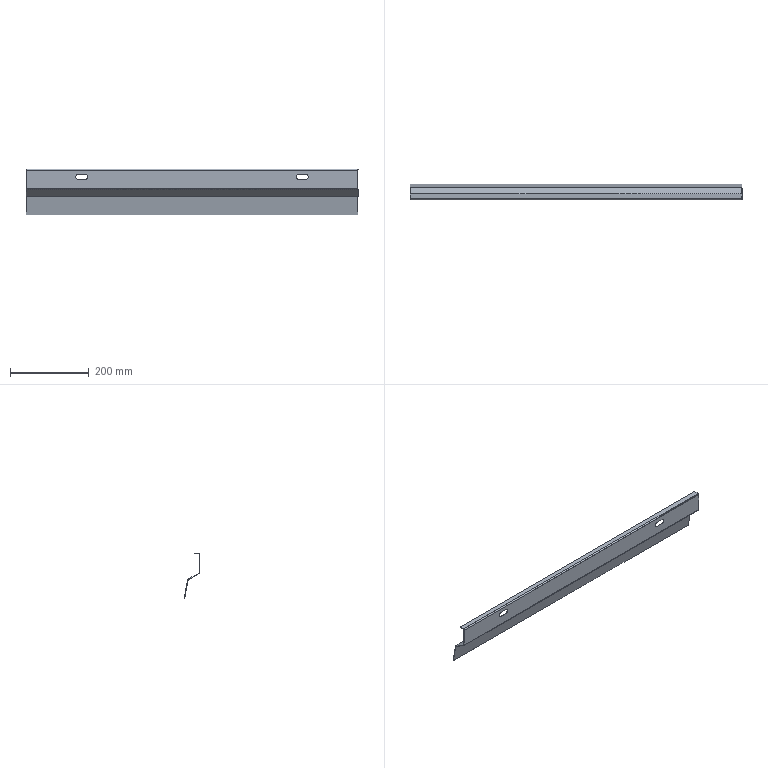Part | SolidWorks | features BaseBody 1 | 1 solid | 26 faces | box 845 x 40.182 x 116.821 mm | volume 185217 mm3 | plane 16 | cylinder 10 | commonest cylinder face diameters 13 x4 3 x3 6 x3
STEP:
#1=CARTESIAN_POINT('',(0.,37.205,-116.821));
#2=VERTEX_POINT('',#1);
#3=CARTESIAN_POINT('',(0.,28.766,-68.959));
#4=VERTEX_POINT('',#3);
#5=CARTESIAN_POINT('',(0.,25.548,-50.712));
#6=DIRECTION('',(0.,-0.1736,0.9848));
#7=VECTOR('',#6,1000.);
#8=LINE('',#5,#7);
#9=EDGE_CURVE('',#2,#4,#8,.T.);
#10=ORIENTED_EDGE('',*,*,#9,.F.);
#11=CARTESIAN_POINT('',(845.,37.205,-116.821));
#12=VERTEX_POINT('',#11);
#13=CARTESIAN_POINT('',(422.5,37.205,-116.821));
#14=DIRECTION('',(-1.,0.,0.));
#15=VECTOR('',#14,1000.);
#16=LINE('',#13,#15);
#17=EDGE_CURVE('',#12,#2,#16,.T.);
#18=ORIENTED_EDGE('',*,*,#17,.F.);
#19=CARTESIAN_POINT('',(845.,28.766,-68.959));
#20=VERTEX_POINT('',#19);
#21=CARTESIAN_POINT('',(845.,25.548,-50.712));
#22=DIRECTION('',(0.,0.1736,-0.9848));
#23=VECTOR('',#22,1000.);
#24=LINE('',#21,#23);
#25=EDGE_CURVE('',#20,#12,#24,.T.);
#26=ORIENTED_EDGE('',*,*,#25,.F.);
#27=CARTESIAN_POINT('',(422.5,28.766,-68.959));
#28=DIRECTION('',(1.,0.,0.));
#29=VECTOR('',#28,1000.);
#30=LINE('',#27,#29);
#31=EDGE_CURVE('',#4,#20,#30,.T.);
#32=ORIENTED_EDGE('',*,*,#31,.F.);
#33=EDGE_LOOP('',(#10,#18,#26,#32));
#34=FACE_OUTER_BOUND('',#33,.T.);
#35=CARTESIAN_POINT('',(422.5,25.548,-50.712));
#36=DIRECTION('',(0.,0.9848,0.1736));
#37=DIRECTION('',(0.,-0.1736,0.9848));
#38=AXIS2_PLACEMENT_3D('',#35,#36,#37);
#39=PLANE('',#38);
#40=ADVANCED_FACE('',(#34),#39,.F.);
#41=CARTESIAN_POINT('',(845.,28.038,-67.92));
#42=VERTEX_POINT('',#41);
#43=CARTESIAN_POINT('',(845.,27.288,-69.219));
#44=DIRECTION('',(-1.,0.,0.));
#45=DIRECTION('',(0.,0.,1.));
#46=AXIS2_PLACEMENT_3D('',#43,#44,#45);
#47=CIRCLE('',#46,1.5);
#48=EDGE_CURVE('',#42,#20,#47,.T.);
#49=ORIENTED_EDGE('',*,*,#48,.F.);
#50=CARTESIAN_POINT('',(0.,28.038,-67.92));
#51=VERTEX_POINT('',#50);
#52=CARTESIAN_POINT('',(422.5,28.038,-67.92));
#53=DIRECTION('',(1.,0.,0.));
#54=VECTOR('',#53,1000.);
#55=LINE('',#52,#54);
#56=EDGE_CURVE('',#51,#42,#55,.T.);
#57=ORIENTED_EDGE('',*,*,#56,.F.);
#58=CARTESIAN_POINT('',(0.,27.288,-69.219));
#59=DIRECTION('',(1.,0.,0.));
#60=DIRECTION('',(0.,0.,1.));
#61=AXIS2_PLACEMENT_3D('',#58,#59,#60);
#62=CIRCLE('',#61,1.5);
#63=EDGE_CURVE('',#4,#51,#62,.T.);
#64=ORIENTED_EDGE('',*,*,#63,.F.);
#65=ORIENTED_EDGE('',*,*,#31,.T.);
#66=EDGE_LOOP('',(#49,#57,#64,#65));
#67=FACE_OUTER_BOUND('',#66,.T.);
#68=CARTESIAN_POINT('',(422.5,27.288,-69.219));
#69=DIRECTION('',(-1.,0.,0.));
#70=DIRECTION('',(0.,0.,1.));
#71=AXIS2_PLACEMENT_3D('',#68,#69,#70);
#72=CYLINDRICAL_SURFACE('',#71,1.5);
#73=ADVANCED_FACE('',(#67),#72,.F.);
#74=CARTESIAN_POINT('',(0.,38.682,-116.561));
#75=VERTEX_POINT('',#74);
#76=CARTESIAN_POINT('',(0.,38.682,-116.561));
#77=DIRECTION('',(0.,-0.9848,-0.1736));
#78=VECTOR('',#77,1000.);
#79=LINE('',#76,#78);
#80=EDGE_CURVE('',#75,#2,#79,.T.);
#81=ORIENTED_EDGE('',*,*,#80,.T.);
#82=ORIENTED_EDGE('',*,*,#9,.T.);
#83=ORIENTED_EDGE('',*,*,#63,.T.);
#84=CARTESIAN_POINT('',(0.,0.,-51.732));
#85=VERTEX_POINT('',#84);
#86=CARTESIAN_POINT('',(0.,13.625,-59.599));
#87=DIRECTION('',(0.,-0.866,0.5));
#88=VECTOR('',#87,1000.);
#89=LINE('',#86,#88);
#90=EDGE_CURVE('',#51,#85,#89,.T.);
#91=ORIENTED_EDGE('',*,*,#90,.T.);
#92=CARTESIAN_POINT('',(0.,-1.5,-49.134));
#93=VERTEX_POINT('',#92);
#94=CARTESIAN_POINT('',(0.,1.5,-49.134));
#95=DIRECTION('',(1.,0.,0.));
#96=DIRECTION('',(0.,0.,-1.));
#97=AXIS2_PLACEMENT_3D('',#94,#95,#96);
#98=CIRCLE('',#97,3.);
#99=EDGE_CURVE('',#93,#85,#98,.T.);
#100=ORIENTED_EDGE('',*,*,#99,.F.);
#101=CARTESIAN_POINT('',(0.,-1.5,-3.));
#102=VERTEX_POINT('',#101);
#103=CARTESIAN_POINT('',(0.,-1.5,-67.129));
#104=DIRECTION('',(0.,0.,1.));
#105=VECTOR('',#104,1000.);
#106=LINE('',#103,#105);
#107=EDGE_CURVE('',#93,#102,#106,.T.);
#108=ORIENTED_EDGE('',*,*,#107,.T.);
#109=CARTESIAN_POINT('',(0.,1.5,0.));
#110=VERTEX_POINT('',#109);
#111=CARTESIAN_POINT('',(0.,1.5,-3.));
#112=DIRECTION('',(1.,0.,0.));
#113=DIRECTION('',(0.,-1.,0.));
#114=AXIS2_PLACEMENT_3D('',#111,#112,#113);
#115=CIRCLE('',#114,3.);
#116=EDGE_CURVE('',#110,#102,#115,.T.);
#117=ORIENTED_EDGE('',*,*,#116,.F.);
#118=CARTESIAN_POINT('',(0.,13.5,0.));
#119=VERTEX_POINT('',#118);
#120=CARTESIAN_POINT('',(0.,5.804,0.));
#121=DIRECTION('',(0.,1.,0.));
#122=VECTOR('',#121,1000.);
#123=LINE('',#120,#122);
#124=EDGE_CURVE('',#110,#119,#123,.T.);
#125=ORIENTED_EDGE('',*,*,#124,.T.);
#126=CARTESIAN_POINT('',(0.,13.5,-1.5));
#127=VERTEX_POINT('',#126);
#128=CARTESIAN_POINT('',(0.,13.5,-1.5));
#129=DIRECTION('',(0.,0.,1.));
#130=VECTOR('',#129,1000.);
#131=LINE('',#128,#130);
#132=EDGE_CURVE('',#127,#119,#131,.T.);
#133=ORIENTED_EDGE('',*,*,#132,.F.);
#134=CARTESIAN_POINT('',(0.,1.5,-1.5));
#135=VERTEX_POINT('',#134);
#136=CARTESIAN_POINT('',(0.,1.5,-1.5));
#137=DIRECTION('',(0.,-1.,0.));
#138=VECTOR('',#137,1000.);
#139=LINE('',#136,#138);
#140=EDGE_CURVE('',#127,#135,#139,.T.);
#141=ORIENTED_EDGE('',*,*,#140,.T.);
#142=CARTESIAN_POINT('',(0.,0.,-3.));
#143=VERTEX_POINT('',#142);
#144=CARTESIAN_POINT('',(0.,1.5,-3.));
#145=DIRECTION('',(1.,0.,0.));
#146=DIRECTION('',(0.,-1.,0.));
#147=AXIS2_PLACEMENT_3D('',#144,#145,#146);
#148=CIRCLE('',#147,1.5);
#149=EDGE_CURVE('',#135,#143,#148,.T.);
#150=ORIENTED_EDGE('',*,*,#149,.T.);
#151=CARTESIAN_POINT('',(0.,0.,-49.134));
#152=VERTEX_POINT('',#151);
#153=CARTESIAN_POINT('',(0.,0.,-85.657));
#154=DIRECTION('',(0.,0.,-1.));
#155=VECTOR('',#154,1000.);
#156=LINE('',#153,#155);
#157=EDGE_CURVE('',#143,#152,#156,.T.);
#158=ORIENTED_EDGE('',*,*,#157,.T.);
#159=CARTESIAN_POINT('',(0.,0.75,-50.433));
#160=VERTEX_POINT('',#159);
#161=CARTESIAN_POINT('',(0.,1.5,-49.134));
#162=DIRECTION('',(1.,0.,0.));
#163=DIRECTION('',(0.,0.,-1.));
#164=AXIS2_PLACEMENT_3D('',#161,#162,#163);
#165=CIRCLE('',#164,1.5);
#166=EDGE_CURVE('',#152,#160,#165,.T.);
#167=ORIENTED_EDGE('',*,*,#166,.T.);
#168=CARTESIAN_POINT('',(0.,28.788,-66.621));
#169=VERTEX_POINT('',#168);
#170=CARTESIAN_POINT('',(0.,0.75,-50.433));
#171=DIRECTION('',(0.,0.866,-0.5));
#172=VECTOR('',#171,1000.);
#173=LINE('',#170,#172);
#174=EDGE_CURVE('',#160,#169,#173,.T.);
#175=ORIENTED_EDGE('',*,*,#174,.T.);
#176=CARTESIAN_POINT('',(0.,30.243,-68.698));
#177=VERTEX_POINT('',#176);
#178=CARTESIAN_POINT('',(0.,27.288,-69.219));
#179=DIRECTION('',(1.,0.,0.));
#180=DIRECTION('',(0.,0.,1.));
#181=AXIS2_PLACEMENT_3D('',#178,#179,#180);
#182=CIRCLE('',#181,3.);
#183=EDGE_CURVE('',#177,#169,#182,.T.);
#184=ORIENTED_EDGE('',*,*,#183,.F.);
#185=CARTESIAN_POINT('',(0.,30.243,-68.698));
#186=DIRECTION('',(0.,0.1736,-0.9848));
#187=VECTOR('',#186,1000.);
#188=LINE('',#185,#187);
#189=EDGE_CURVE('',#177,#75,#188,.T.);
#190=ORIENTED_EDGE('',*,*,#189,.T.);
#191=EDGE_LOOP('',(#81,#82,#83,#91,#100,#108,#117,#125,#133,#141,#150,#158,#167,#175,#184,#190));
#192=FACE_OUTER_BOUND('',#191,.T.);
#193=CARTESIAN_POINT('',(0.,28.766,-68.959));
#194=DIRECTION('',(-1.,0.,0.));
#195=DIRECTION('',(0.,0.,1.));
#196=AXIS2_PLACEMENT_3D('',#193,#194,#195);
#197=PLANE('',#196);
#198=ADVANCED_FACE('',(#192),#197,.T.);
#199=ORIENTED_EDGE('',*,*,#17,.T.);
#200=ORIENTED_EDGE('',*,*,#80,.F.);
#201=CARTESIAN_POINT('',(845.,38.682,-116.561));
#202=VERTEX_POINT('',#201);
#203=CARTESIAN_POINT('',(0.,38.682,-116.561));
#204=DIRECTION('',(1.,0.,0.));
#205=VECTOR('',#204,1000.);
#206=LINE('',#203,#205);
#207=EDGE_CURVE('',#75,#202,#206,.T.);
#208=ORIENTED_EDGE('',*,*,#207,.T.);
#209=CARTESIAN_POINT('',(845.,37.205,-116.821));
#210=DIRECTION('',(0.,-0.9848,-0.1736));
#211=VECTOR('',#210,1000.);
#212=LINE('',#209,#211);
#213=EDGE_CURVE('',#202,#12,#212,.T.);
#214=ORIENTED_EDGE('',*,*,#213,.T.);
#215=EDGE_LOOP('',(#199,#200,#208,#214));
#216=FACE_OUTER_BOUND('',#215,.T.);
#217=CARTESIAN_POINT('',(0.,37.205,-116.821));
#218=DIRECTION('',(0.,0.1736,-0.9848));
#219=DIRECTION('',(0.,0.9848,0.1736));
#220=AXIS2_PLACEMENT_3D('',#217,#218,#219);
#221=PLANE('',#220);
#222=ADVANCED_FACE('',(#216),#221,.T.);
#223=ORIENTED_EDGE('',*,*,#213,.F.);
#224=CARTESIAN_POINT('',(845.,30.243,-68.698));
#225=VERTEX_POINT('',#224);
#226=CARTESIAN_POINT('',(845.,38.682,-116.561));
#227=DIRECTION('',(0.,-0.1736,0.9848));
#228=VECTOR('',#227,1000.);
#229=LINE('',#226,#228);
#230=EDGE_CURVE('',#202,#225,#229,.T.);
#231=ORIENTED_EDGE('',*,*,#230,.T.);
#232=CARTESIAN_POINT('',(845.,28.788,-66.621));
#233=VERTEX_POINT('',#232);
#234=CARTESIAN_POINT('',(845.,27.288,-69.219));
#235=DIRECTION('',(-1.,0.,0.));
#236=DIRECTION('',(0.,0.,1.));
#237=AXIS2_PLACEMENT_3D('',#234,#235,#236);
#238=CIRCLE('',#237,3.);
#239=EDGE_CURVE('',#233,#225,#238,.T.);
#240=ORIENTED_EDGE('',*,*,#239,.F.);
#241=CARTESIAN_POINT('',(845.,0.75,-50.433));
#242=VERTEX_POINT('',#241);
#243=CARTESIAN_POINT('',(845.,28.788,-66.621));
#244=DIRECTION('',(0.,-0.866,0.5));
#245=VECTOR('',#244,1000.);
#246=LINE('',#243,#245);
#247=EDGE_CURVE('',#233,#242,#246,.T.);
#248=ORIENTED_EDGE('',*,*,#247,.T.);
#249=CARTESIAN_POINT('',(845.,0.,-49.134));
#250=VERTEX_POINT('',#249);
#251=CARTESIAN_POINT('',(845.,1.5,-49.134));
#252=DIRECTION('',(-1.,0.,0.));
#253=DIRECTION('',(0.,0.,-1.));
#254=AXIS2_PLACEMENT_3D('',#251,#252,#253);
#255=CIRCLE('',#254,1.5);
#256=EDGE_CURVE('',#242,#250,#255,.T.);
#257=ORIENTED_EDGE('',*,*,#256,.T.);
#258=CARTESIAN_POINT('',(845.,0.,-3.));
#259=VERTEX_POINT('',#258);
#260=CARTESIAN_POINT('',(845.,0.,-49.134));
#261=DIRECTION('',(0.,0.,1.));
#262=VECTOR('',#261,1000.);
#263=LINE('',#260,#262);
#264=EDGE_CURVE('',#250,#259,#263,.T.);
#265=ORIENTED_EDGE('',*,*,#264,.T.);
#266=CARTESIAN_POINT('',(845.,1.5,-1.5));
#267=VERTEX_POINT('',#266);
#268=CARTESIAN_POINT('',(845.,1.5,-3.));
#269=DIRECTION('',(-1.,0.,0.));
#270=DIRECTION('',(0.,-1.,0.));
#271=AXIS2_PLACEMENT_3D('',#268,#269,#270);
#272=CIRCLE('',#271,1.5);
#273=EDGE_CURVE('',#259,#267,#272,.T.);
#274=ORIENTED_EDGE('',*,*,#273,.T.);
#275=CARTESIAN_POINT('',(845.,13.5,-1.5));
#276=VERTEX_POINT('',#275);
#277=CARTESIAN_POINT('',(845.,1.5,-1.5));
#278=DIRECTION('',(0.,1.,0.));
#279=VECTOR('',#278,1000.);
#280=LINE('',#277,#279);
#281=EDGE_CURVE('',#267,#276,#280,.T.);
#282=ORIENTED_EDGE('',*,*,#281,.T.);
#283=CARTESIAN_POINT('',(845.,13.5,0.));
#284=VERTEX_POINT('',#283);
#285=CARTESIAN_POINT('',(845.,13.5,-1.5));
#286=DIRECTION('',(0.,0.,1.));
#287=VECTOR('',#286,1000.);
#288=LINE('',#285,#287);
#289=EDGE_CURVE('',#276,#284,#288,.T.);
#290=ORIENTED_EDGE('',*,*,#289,.T.);
#291=CARTESIAN_POINT('',(845.,1.5,0.));
#292=VERTEX_POINT('',#291);
#293=CARTESIAN_POINT('',(845.,5.804,0.));
#294=DIRECTION('',(0.,-1.,0.));
#295=VECTOR('',#294,1000.);
#296=LINE('',#293,#295);
#297=EDGE_CURVE('',#284,#292,#296,.T.);
#298=ORIENTED_EDGE('',*,*,#297,.T.);
#299=CARTESIAN_POINT('',(845.,-1.5,-3.));
#300=VERTEX_POINT('',#299);
#301=CARTESIAN_POINT('',(845.,1.5,-3.));
#302=DIRECTION('',(-1.,0.,0.));
#303=DIRECTION('',(0.,-1.,0.));
#304=AXIS2_PLACEMENT_3D('',#301,#302,#303);
#305=CIRCLE('',#304,3.);
#306=EDGE_CURVE('',#300,#292,#305,.T.);
#307=ORIENTED_EDGE('',*,*,#306,.F.);
#308=CARTESIAN_POINT('',(845.,-1.5,-49.134));
#309=VERTEX_POINT('',#308);
#310=CARTESIAN_POINT('',(845.,-1.5,-67.129));
#311=DIRECTION('',(0.,0.,-1.));
#312=VECTOR('',#311,1000.);
#313=LINE('',#310,#312);
#314=EDGE_CURVE('',#300,#309,#313,.T.);
#315=ORIENTED_EDGE('',*,*,#314,.T.);
#316=CARTESIAN_POINT('',(845.,0.,-51.732));
#317=VERTEX_POINT('',#316);
#318=CARTESIAN_POINT('',(845.,1.5,-49.134));
#319=DIRECTION('',(-1.,0.,0.));
#320=DIRECTION('',(0.,0.,-1.));
#321=AXIS2_PLACEMENT_3D('',#318,#319,#320);
#322=CIRCLE('',#321,3.);
#323=EDGE_CURVE('',#317,#309,#322,.T.);
#324=ORIENTED_EDGE('',*,*,#323,.F.);
#325=CARTESIAN_POINT('',(845.,13.625,-59.599));
#326=DIRECTION('',(0.,0.866,-0.5));
#327=VECTOR('',#326,1000.);
#328=LINE('',#325,#327);
#329=EDGE_CURVE('',#317,#42,#328,.T.);
#330=ORIENTED_EDGE('',*,*,#329,.T.);
#331=ORIENTED_EDGE('',*,*,#48,.T.);
#332=ORIENTED_EDGE('',*,*,#25,.T.);
#333=EDGE_LOOP('',(#223,#231,#240,#248,#257,#265,#274,#282,#290,#298,#307,#315,#324,#330,#331,#332));
#334=FACE_OUTER_BOUND('',#333,.T.);
#335=CARTESIAN_POINT('',(845.,22.424,-32.991));
#336=DIRECTION('',(1.,0.,0.));
#337=DIRECTION('',(0.,0.,-1.));
#338=AXIS2_PLACEMENT_3D('',#335,#336,#337);
#339=PLANE('',#338);
#340=ADVANCED_FACE('',(#334),#339,.T.);
#341=ORIENTED_EDGE('',*,*,#329,.F.);
#342=CARTESIAN_POINT('',(422.5,0.,-51.732));
#343=DIRECTION('',(1.,0.,0.));
#344=VECTOR('',#343,1000.);
#345=LINE('',#342,#344);
#346=EDGE_CURVE('',#85,#317,#345,.T.);
#347=ORIENTED_EDGE('',*,*,#346,.F.);
#348=ORIENTED_EDGE('',*,*,#90,.F.);
#349=ORIENTED_EDGE('',*,*,#56,.T.);
#350=EDGE_LOOP('',(#341,#347,#348,#349));
#351=FACE_OUTER_BOUND('',#350,.T.);
#352=CARTESIAN_POINT('',(422.5,13.625,-59.599));
#353=DIRECTION('',(0.,0.5,0.866));
#354=DIRECTION('',(0.,-0.866,0.5));
#355=AXIS2_PLACEMENT_3D('',#352,#353,#354);
#356=PLANE('',#355);
#357=ADVANCED_FACE('',(#351),#356,.F.);
#358=ORIENTED_EDGE('',*,*,#207,.F.);
#359=ORIENTED_EDGE('',*,*,#189,.F.);
#360=CARTESIAN_POINT('',(422.5,30.243,-68.698));
#361=DIRECTION('',(1.,0.,0.));
#362=VECTOR('',#361,1000.);
#363=LINE('',#360,#362);
#364=EDGE_CURVE('',#177,#225,#363,.T.);
#365=ORIENTED_EDGE('',*,*,#364,.T.);
#366=ORIENTED_EDGE('',*,*,#230,.F.);
#367=EDGE_LOOP('',(#358,#359,#365,#366));
#368=FACE_OUTER_BOUND('',#367,.T.);
#369=CARTESIAN_POINT('',(422.5,27.026,-50.452));
#370=DIRECTION('',(0.,0.9848,0.1736));
#371=DIRECTION('',(0.,-0.1736,0.9848));
#372=AXIS2_PLACEMENT_3D('',#369,#370,#371);
#373=PLANE('',#372);
#374=ADVANCED_FACE('',(#368),#373,.T.);
#375=CARTESIAN_POINT('',(422.5,-1.5,-49.134));
#376=DIRECTION('',(-1.,0.,0.));
#377=VECTOR('',#376,1000.);
#378=LINE('',#375,#377);
#379=EDGE_CURVE('',#309,#93,#378,.T.);
#380=ORIENTED_EDGE('',*,*,#379,.T.);
#381=ORIENTED_EDGE('',*,*,#99,.T.);
#382=ORIENTED_EDGE('',*,*,#346,.T.);
#383=ORIENTED_EDGE('',*,*,#323,.T.);
#384=EDGE_LOOP('',(#380,#381,#382,#383));
#385=FACE_OUTER_BOUND('',#384,.T.);
#386=CARTESIAN_POINT('',(422.5,1.5,-49.134));
#387=DIRECTION('',(1.,0.,0.));
#388=DIRECTION('',(0.,0.,-1.));
#389=AXIS2_PLACEMENT_3D('',#386,#387,#388);
#390=CYLINDRICAL_SURFACE('',#389,3.);
#391=ADVANCED_FACE('',(#385),#390,.T.);
#392=CARTESIAN_POINT('',(422.5,28.788,-66.621));
#393=DIRECTION('',(1.,0.,0.));
#394=VECTOR('',#393,1000.);
#395=LINE('',#392,#394);
#396=EDGE_CURVE('',#169,#233,#395,.T.);
#397=ORIENTED_EDGE('',*,*,#396,.T.);
#398=ORIENTED_EDGE('',*,*,#239,.T.);
#399=ORIENTED_EDGE('',*,*,#364,.F.);
#400=ORIENTED_EDGE('',*,*,#183,.T.);
#401=EDGE_LOOP('',(#397,#398,#399,#400));
#402=FACE_OUTER_BOUND('',#401,.T.);
#403=CARTESIAN_POINT('',(422.5,27.288,-69.219));
#404=DIRECTION('',(-1.,0.,0.));
#405=DIRECTION('',(0.,0.,1.));
#406=AXIS2_PLACEMENT_3D('',#403,#404,#405);
#407=CYLINDRICAL_SURFACE('',#406,3.);
#408=ADVANCED_FACE('',(#402),#407,.T.);
#409=CARTESIAN_POINT('',(422.5,0.75,-50.433));
#410=DIRECTION('',(1.,0.,0.));
#411=VECTOR('',#410,1000.);
#412=LINE('',#409,#411);
#413=EDGE_CURVE('',#160,#242,#412,.T.);
#414=ORIENTED_EDGE('',*,*,#413,.T.);
#415=ORIENTED_EDGE('',*,*,#247,.F.);
#416=ORIENTED_EDGE('',*,*,#396,.F.);
#417=ORIENTED_EDGE('',*,*,#174,.F.);
#418=EDGE_LOOP('',(#414,#415,#416,#417));
#419=FACE_OUTER_BOUND('',#418,.T.);
#420=CARTESIAN_POINT('',(422.5,14.375,-58.3));
#421=DIRECTION('',(0.,0.5,0.866));
#422=DIRECTION('',(0.,-0.866,0.5));
#423=AXIS2_PLACEMENT_3D('',#420,#421,#422);
#424=PLANE('',#423);
#425=ADVANCED_FACE('',(#419),#424,.T.);
#426=CARTESIAN_POINT('',(695.,-1.5,-26.5));
#427=VERTEX_POINT('',#426);
#428=CARTESIAN_POINT('',(712.,-1.5,-26.5));
#429=VERTEX_POINT('',#428);
#430=CARTESIAN_POINT('',(422.5,-1.5,-26.5));
#431=DIRECTION('',(1.,0.,0.));
#432=VECTOR('',#431,1000.);
#433=LINE('',#430,#432);
#434=EDGE_CURVE('',#427,#429,#433,.T.);
#435=ORIENTED_EDGE('',*,*,#434,.F.);
#436=CARTESIAN_POINT('',(695.,-1.5,-13.5));
#437=VERTEX_POINT('',#436);
#438=CARTESIAN_POINT('',(695.,-1.5,-20.));
#439=DIRECTION('',(0.,-1.,0.));
#440=DIRECTION('',(0.,0.,1.));
#441=AXIS2_PLACEMENT_3D('',#438,#439,#440);
#442=CIRCLE('',#441,6.5);
#443=EDGE_CURVE('',#437,#427,#442,.T.);
#444=ORIENTED_EDGE('',*,*,#443,.F.);
#445=CARTESIAN_POINT('',(712.,-1.5,-13.5));
#446=VERTEX_POINT('',#445);
#447=CARTESIAN_POINT('',(422.5,-1.5,-13.5));
#448=DIRECTION('',(-1.,0.,0.));
#449=VECTOR('',#448,1000.);
#450=LINE('',#447,#449);
#451=EDGE_CURVE('',#446,#437,#450,.T.);
#452=ORIENTED_EDGE('',*,*,#451,.F.);
#453=CARTESIAN_POINT('',(712.,-1.5,-20.));
#454=DIRECTION('',(0.,-1.,0.));
#455=DIRECTION('',(0.,0.,1.));
#456=AXIS2_PLACEMENT_3D('',#453,#454,#455);
#457=CIRCLE('',#456,6.5);
#458=EDGE_CURVE('',#429,#446,#457,.T.);
#459=ORIENTED_EDGE('',*,*,#458,.F.);
#460=EDGE_LOOP('',(#435,#444,#452,#459));
#461=FACE_BOUND('',#460,.T.);
#462=CARTESIAN_POINT('',(133.,-1.5,-26.5));
#463=VERTEX_POINT('',#462);
#464=CARTESIAN_POINT('',(150.,-1.5,-26.5));
#465=VERTEX_POINT('',#464);
#466=CARTESIAN_POINT('',(422.5,-1.5,-26.5));
#467=DIRECTION('',(1.,0.,0.));
#468=VECTOR('',#467,1000.);
#469=LINE('',#466,#468);
#470=EDGE_CURVE('',#463,#465,#469,.T.);
#471=ORIENTED_EDGE('',*,*,#470,.F.);
#472=CARTESIAN_POINT('',(133.,-1.5,-13.5));
#473=VERTEX_POINT('',#472);
#474=CARTESIAN_POINT('',(133.,-1.5,-20.));
#475=DIRECTION('',(0.,-1.,0.));
#476=DIRECTION('',(0.,0.,1.));
#477=AXIS2_PLACEMENT_3D('',#474,#475,#476);
#478=CIRCLE('',#477,6.5);
#479=EDGE_CURVE('',#473,#463,#478,.T.);
#480=ORIENTED_EDGE('',*,*,#479,.F.);
#481=CARTESIAN_POINT('',(150.,-1.5,-13.5));
#482=VERTEX_POINT('',#481);
#483=CARTESIAN_POINT('',(422.5,-1.5,-13.5));
#484=DIRECTION('',(-1.,0.,0.));
#485=VECTOR('',#484,1000.);
#486=LINE('',#483,#485);
#487=EDGE_CURVE('',#482,#473,#486,.T.);
#488=ORIENTED_EDGE('',*,*,#487,.F.);
#489=CARTESIAN_POINT('',(150.,-1.5,-20.));
#490=DIRECTION('',(0.,-1.,0.));
#491=DIRECTION('',(0.,0.,1.));
#492=AXIS2_PLACEMENT_3D('',#489,#490,#491);
#493=CIRCLE('',#492,6.5);
#494=EDGE_CURVE('',#465,#482,#493,.T.);
#495=ORIENTED_EDGE('',*,*,#494,.F.);
#496=EDGE_LOOP('',(#471,#480,#488,#495));
#497=FACE_BOUND('',#496,.T.);
#498=ORIENTED_EDGE('',*,*,#107,.F.);
#499=ORIENTED_EDGE('',*,*,#379,.F.);
#500=ORIENTED_EDGE('',*,*,#314,.F.);
#501=CARTESIAN_POINT('',(422.5,-1.5,-3.));
#502=DIRECTION('',(1.,0.,0.));
#503=VECTOR('',#502,1000.);
#504=LINE('',#501,#503);
#505=EDGE_CURVE('',#102,#300,#504,.T.);
#506=ORIENTED_EDGE('',*,*,#505,.F.);
#507=EDGE_LOOP('',(#498,#499,#500,#506));
#508=FACE_OUTER_BOUND('',#507,.T.);
#509=CARTESIAN_POINT('',(422.5,-1.5,-67.129));
#510=DIRECTION('',(0.,1.,0.));
#511=DIRECTION('',(0.,0.,1.));
#512=AXIS2_PLACEMENT_3D('',#509,#510,#511);
#513=PLANE('',#512);
#514=ADVANCED_FACE('',(#461,#497,#508),#513,.F.);
#515=ORIENTED_EDGE('',*,*,#166,.F.);
#516=CARTESIAN_POINT('',(422.5,0.,-49.134));
#517=DIRECTION('',(-1.,0.,0.));
#518=VECTOR('',#517,1000.);
#519=LINE('',#516,#518);
#520=EDGE_CURVE('',#250,#152,#519,.T.);
#521=ORIENTED_EDGE('',*,*,#520,.F.);
#522=ORIENTED_EDGE('',*,*,#256,.F.);
#523=ORIENTED_EDGE('',*,*,#413,.F.);
#524=EDGE_LOOP('',(#515,#521,#522,#523));
#525=FACE_OUTER_BOUND('',#524,.T.);
#526=CARTESIAN_POINT('',(422.5,1.5,-49.134));
#527=DIRECTION('',(1.,0.,0.));
#528=DIRECTION('',(0.,0.,-1.));
#529=AXIS2_PLACEMENT_3D('',#526,#527,#528);
#530=CYLINDRICAL_SURFACE('',#529,1.5);
#531=ADVANCED_FACE('',(#525),#530,.F.);
#532=CARTESIAN_POINT('',(712.,0.,-13.5));
#533=VERTEX_POINT('',#532);
#534=CARTESIAN_POINT('',(712.,-1.5,-13.5));
#535=DIRECTION('',(0.,-1.,0.));
#536=VECTOR('',#535,1000.);
#537=LINE('',#534,#536);
#538=EDGE_CURVE('',#533,#446,#537,.T.);
#539=ORIENTED_EDGE('',*,*,#538,.F.);
#540=CARTESIAN_POINT('',(712.,0.,-26.5));
#541=VERTEX_POINT('',#540);
#542=CARTESIAN_POINT('',(712.,0.,-20.));
#543=DIRECTION('',(0.,-1.,0.));
#544=DIRECTION('',(0.,0.,1.));
#545=AXIS2_PLACEMENT_3D('',#542,#543,#544);
#546=CIRCLE('',#545,6.5);
#547=EDGE_CURVE('',#541,#533,#546,.T.);
#548=ORIENTED_EDGE('',*,*,#547,.F.);
#549=CARTESIAN_POINT('',(712.,-1.5,-26.5));
#550=DIRECTION('',(0.,1.,0.));
#551=VECTOR('',#550,1000.);
#552=LINE('',#549,#551);
#553=EDGE_CURVE('',#429,#541,#552,.T.);
#554=ORIENTED_EDGE('',*,*,#553,.F.);
#555=ORIENTED_EDGE('',*,*,#458,.T.);
#556=EDGE_LOOP('',(#539,#548,#554,#555));
#557=FACE_OUTER_BOUND('',#556,.T.);
#558=CARTESIAN_POINT('',(712.,-1.5,-20.));
#559=DIRECTION('',(0.,1.,0.));
#560=DIRECTION('',(0.,0.,1.));
#561=AXIS2_PLACEMENT_3D('',#558,#559,#560);
#562=CYLINDRICAL_SURFACE('',#561,6.5);
#563=ADVANCED_FACE('',(#557),#562,.F.);
#564=ORIENTED_EDGE('',*,*,#553,.T.);
#565=CARTESIAN_POINT('',(695.,0.,-26.5));
#566=VERTEX_POINT('',#565);
#567=CARTESIAN_POINT('',(712.,0.,-26.5));
#568=DIRECTION('',(1.,0.,0.));
#569=VECTOR('',#568,1000.);
#570=LINE('',#567,#569);
#571=EDGE_CURVE('',#566,#541,#570,.T.);
#572=ORIENTED_EDGE('',*,*,#571,.F.);
#573=CARTESIAN_POINT('',(695.,-1.5,-26.5));
#574=DIRECTION('',(0.,1.,0.));
#575=VECTOR('',#574,1000.);
#576=LINE('',#573,#575);
#577=EDGE_CURVE('',#427,#566,#576,.T.);
#578=ORIENTED_EDGE('',*,*,#577,.F.);
#579=ORIENTED_EDGE('',*,*,#434,.T.);
#580=EDGE_LOOP('',(#564,#572,#578,#579));
#581=FACE_OUTER_BOUND('',#580,.T.);
#582=CARTESIAN_POINT('',(712.,-1.5,-26.5));
#583=DIRECTION('',(0.,0.,-1.));
#584=DIRECTION('',(-1.,0.,0.));
#585=AXIS2_PLACEMENT_3D('',#582,#583,#584);
#586=PLANE('',#585);
#587=ADVANCED_FACE('',(#581),#586,.F.);
#588=ORIENTED_EDGE('',*,*,#577,.T.);
#589=CARTESIAN_POINT('',(695.,0.,-13.5));
#590=VERTEX_POINT('',#589);
#591=CARTESIAN_POINT('',(695.,0.,-20.));
#592=DIRECTION('',(0.,-1.,0.));
#593=DIRECTION('',(0.,0.,1.));
#594=AXIS2_PLACEMENT_3D('',#591,#592,#593);
#595=CIRCLE('',#594,6.5);
#596=EDGE_CURVE('',#590,#566,#595,.T.);
#597=ORIENTED_EDGE('',*,*,#596,.F.);
#598=CARTESIAN_POINT('',(695.,-1.5,-13.5));
#599=DIRECTION('',(0.,1.,0.));
#600=VECTOR('',#599,1000.);
#601=LINE('',#598,#600);
#602=EDGE_CURVE('',#437,#590,#601,.T.);
#603=ORIENTED_EDGE('',*,*,#602,.F.);
#604=ORIENTED_EDGE('',*,*,#443,.T.);
#605=EDGE_LOOP('',(#588,#597,#603,#604));
#606=FACE_OUTER_BOUND('',#605,.T.);
#607=CARTESIAN_POINT('',(695.,-1.5,-20.));
#608=DIRECTION('',(0.,1.,0.));
#609=DIRECTION('',(0.,0.,1.));
#610=AXIS2_PLACEMENT_3D('',#607,#608,#609);
#611=CYLINDRICAL_SURFACE('',#610,6.5);
#612=ADVANCED_FACE('',(#606),#611,.F.);
#613=ORIENTED_EDGE('',*,*,#602,.T.);
#614=CARTESIAN_POINT('',(695.,0.,-13.5));
#615=DIRECTION('',(-1.,0.,0.));
#616=VECTOR('',#615,1000.);
#617=LINE('',#614,#616);
#618=EDGE_CURVE('',#533,#590,#617,.T.);
#619=ORIENTED_EDGE('',*,*,#618,.F.);
#620=ORIENTED_EDGE('',*,*,#538,.T.);
#621=ORIENTED_EDGE('',*,*,#451,.T.);
#622=EDGE_LOOP('',(#613,#619,#620,#621));
#623=FACE_OUTER_BOUND('',#622,.T.);
#624=CARTESIAN_POINT('',(695.,-1.5,-13.5));
#625=DIRECTION('',(0.,0.,1.));
#626=DIRECTION('',(1.,0.,0.));
#627=AXIS2_PLACEMENT_3D('',#624,#625,#626);
#628=PLANE('',#627);
#629=ADVANCED_FACE('',(#623),#628,.F.);
#630=CARTESIAN_POINT('',(150.,0.,-13.5));
#631=VERTEX_POINT('',#630);
#632=CARTESIAN_POINT('',(150.,-1.5,-13.5));
#633=DIRECTION('',(0.,-1.,0.));
#634=VECTOR('',#633,1000.);
#635=LINE('',#632,#634);
#636=EDGE_CURVE('',#631,#482,#635,.T.);
#637=ORIENTED_EDGE('',*,*,#636,.F.);
#638=CARTESIAN_POINT('',(150.,0.,-26.5));
#639=VERTEX_POINT('',#638);
#640=CARTESIAN_POINT('',(150.,0.,-20.));
#641=DIRECTION('',(0.,-1.,0.));
#642=DIRECTION('',(0.,0.,1.));
#643=AXIS2_PLACEMENT_3D('',#640,#641,#642);
#644=CIRCLE('',#643,6.5);
#645=EDGE_CURVE('',#639,#631,#644,.T.);
#646=ORIENTED_EDGE('',*,*,#645,.F.);
#647=CARTESIAN_POINT('',(150.,-1.5,-26.5));
#648=DIRECTION('',(0.,1.,0.));
#649=VECTOR('',#648,1000.);
#650=LINE('',#647,#649);
#651=EDGE_CURVE('',#465,#639,#650,.T.);
#652=ORIENTED_EDGE('',*,*,#651,.F.);
#653=ORIENTED_EDGE('',*,*,#494,.T.);
#654=EDGE_LOOP('',(#637,#646,#652,#653));
#655=FACE_OUTER_BOUND('',#654,.T.);
#656=CARTESIAN_POINT('',(150.,-1.5,-20.));
#657=DIRECTION('',(0.,1.,0.));
#658=DIRECTION('',(0.,0.,1.));
#659=AXIS2_PLACEMENT_3D('',#656,#657,#658);
#660=CYLINDRICAL_SURFACE('',#659,6.5);
#661=ADVANCED_FACE('',(#655),#660,.F.);
#662=ORIENTED_EDGE('',*,*,#651,.T.);
#663=CARTESIAN_POINT('',(133.,0.,-26.5));
#664=VERTEX_POINT('',#663);
#665=CARTESIAN_POINT('',(150.,0.,-26.5));
#666=DIRECTION('',(1.,0.,0.));
#667=VECTOR('',#666,1000.);
#668=LINE('',#665,#667);
#669=EDGE_CURVE('',#664,#639,#668,.T.);
#670=ORIENTED_EDGE('',*,*,#669,.F.);
#671=CARTESIAN_POINT('',(133.,-1.5,-26.5));
#672=DIRECTION('',(0.,1.,0.));
#673=VECTOR('',#672,1000.);
#674=LINE('',#671,#673);
#675=EDGE_CURVE('',#463,#664,#674,.T.);
#676=ORIENTED_EDGE('',*,*,#675,.F.);
#677=ORIENTED_EDGE('',*,*,#470,.T.);
#678=EDGE_LOOP('',(#662,#670,#676,#677));
#679=FACE_OUTER_BOUND('',#678,.T.);
#680=CARTESIAN_POINT('',(150.,-1.5,-26.5));
#681=DIRECTION('',(0.,0.,-1.));
#682=DIRECTION('',(-1.,0.,0.));
#683=AXIS2_PLACEMENT_3D('',#680,#681,#682);
#684=PLANE('',#683);
#685=ADVANCED_FACE('',(#679),#684,.F.);
#686=ORIENTED_EDGE('',*,*,#675,.T.);
#687=CARTESIAN_POINT('',(133.,0.,-13.5));
#688=VERTEX_POINT('',#687);
#689=CARTESIAN_POINT('',(133.,0.,-20.));
#690=DIRECTION('',(0.,-1.,0.));
#691=DIRECTION('',(0.,0.,1.));
#692=AXIS2_PLACEMENT_3D('',#689,#690,#691);
#693=CIRCLE('',#692,6.5);
#694=EDGE_CURVE('',#688,#664,#693,.T.);
#695=ORIENTED_EDGE('',*,*,#694,.F.);
#696=CARTESIAN_POINT('',(133.,-1.5,-13.5));
#697=DIRECTION('',(0.,1.,0.));
#698=VECTOR('',#697,1000.);
#699=LINE('',#696,#698);
#700=EDGE_CURVE('',#473,#688,#699,.T.);
#701=ORIENTED_EDGE('',*,*,#700,.F.);
#702=ORIENTED_EDGE('',*,*,#479,.T.);
#703=EDGE_LOOP('',(#686,#695,#701,#702));
#704=FACE_OUTER_BOUND('',#703,.T.);
#705=CARTESIAN_POINT('',(133.,-1.5,-20.));
#706=DIRECTION('',(0.,1.,0.));
#707=DIRECTION('',(0.,0.,1.));
#708=AXIS2_PLACEMENT_3D('',#705,#706,#707);
#709=CYLINDRICAL_SURFACE('',#708,6.5);
#710=ADVANCED_FACE('',(#704),#709,.F.);
#711=ORIENTED_EDGE('',*,*,#700,.T.);
#712=CARTESIAN_POINT('',(133.,0.,-13.5));
#713=DIRECTION('',(-1.,0.,0.));
#714=VECTOR('',#713,1000.);
#715=LINE('',#712,#714);
#716=EDGE_CURVE('',#631,#688,#715,.T.);
#717=ORIENTED_EDGE('',*,*,#716,.F.);
#718=ORIENTED_EDGE('',*,*,#636,.T.);
#719=ORIENTED_EDGE('',*,*,#487,.T.);
#720=EDGE_LOOP('',(#711,#717,#718,#719));
#721=FACE_OUTER_BOUND('',#720,.T.);
#722=CARTESIAN_POINT('',(133.,-1.5,-13.5));
#723=DIRECTION('',(0.,0.,1.));
#724=DIRECTION('',(1.,0.,0.));
#725=AXIS2_PLACEMENT_3D('',#722,#723,#724);
#726=PLANE('',#725);
#727=ADVANCED_FACE('',(#721),#726,.F.);
#728=ORIENTED_EDGE('',*,*,#505,.T.);
#729=ORIENTED_EDGE('',*,*,#306,.T.);
#730=CARTESIAN_POINT('',(422.5,1.5,0.));
#731=DIRECTION('',(-1.,0.,0.));
#732=VECTOR('',#731,1000.);
#733=LINE('',#730,#732);
#734=EDGE_CURVE('',#292,#110,#733,.T.);
#735=ORIENTED_EDGE('',*,*,#734,.T.);
#736=ORIENTED_EDGE('',*,*,#116,.T.);
#737=EDGE_LOOP('',(#728,#729,#735,#736));
#738=FACE_OUTER_BOUND('',#737,.T.);
#739=CARTESIAN_POINT('',(422.5,1.5,-3.));
#740=DIRECTION('',(-1.,0.,0.));
#741=DIRECTION('',(0.,-1.,0.));
#742=AXIS2_PLACEMENT_3D('',#739,#740,#741);
#743=CYLINDRICAL_SURFACE('',#742,3.);
#744=ADVANCED_FACE('',(#738),#743,.T.);
#745=ORIENTED_EDGE('',*,*,#596,.T.);
#746=ORIENTED_EDGE('',*,*,#571,.T.);
#747=ORIENTED_EDGE('',*,*,#547,.T.);
#748=ORIENTED_EDGE('',*,*,#618,.T.);
#749=EDGE_LOOP('',(#745,#746,#747,#748));
#750=FACE_BOUND('',#749,.T.);
#751=ORIENTED_EDGE('',*,*,#694,.T.);
#752=ORIENTED_EDGE('',*,*,#669,.T.);
#753=ORIENTED_EDGE('',*,*,#645,.T.);
#754=ORIENTED_EDGE('',*,*,#716,.T.);
#755=EDGE_LOOP('',(#751,#752,#753,#754));
#756=FACE_BOUND('',#755,.T.);
#757=ORIENTED_EDGE('',*,*,#520,.T.);
#758=ORIENTED_EDGE('',*,*,#157,.F.);
#759=CARTESIAN_POINT('',(422.5,0.,-3.));
#760=DIRECTION('',(1.,0.,0.));
#761=VECTOR('',#760,1000.);
#762=LINE('',#759,#761);
#763=EDGE_CURVE('',#143,#259,#762,.T.);
#764=ORIENTED_EDGE('',*,*,#763,.T.);
#765=ORIENTED_EDGE('',*,*,#264,.F.);
#766=EDGE_LOOP('',(#757,#758,#764,#765));
#767=FACE_OUTER_BOUND('',#766,.T.);
#768=CARTESIAN_POINT('',(422.5,0.,-67.129));
#769=DIRECTION('',(0.,1.,0.));
#770=DIRECTION('',(0.,0.,1.));
#771=AXIS2_PLACEMENT_3D('',#768,#769,#770);
#772=PLANE('',#771);
#773=ADVANCED_FACE('',(#750,#756,#767),#772,.T.);
#774=ORIENTED_EDGE('',*,*,#297,.F.);
#775=CARTESIAN_POINT('',(422.5,13.5,0.));
#776=DIRECTION('',(1.,0.,0.));
#777=VECTOR('',#776,1000.);
#778=LINE('',#775,#777);
#779=EDGE_CURVE('',#119,#284,#778,.T.);
#780=ORIENTED_EDGE('',*,*,#779,.F.);
#781=ORIENTED_EDGE('',*,*,#124,.F.);
#782=ORIENTED_EDGE('',*,*,#734,.F.);
#783=EDGE_LOOP('',(#774,#780,#781,#782));
#784=FACE_OUTER_BOUND('',#783,.T.);
#785=CARTESIAN_POINT('',(422.5,5.804,0.));
#786=DIRECTION('',(0.,0.,-1.));
#787=DIRECTION('',(0.,1.,0.));
#788=AXIS2_PLACEMENT_3D('',#785,#786,#787);
#789=PLANE('',#788);
#790=ADVANCED_FACE('',(#784),#789,.F.);
#791=ORIENTED_EDGE('',*,*,#273,.F.);
#792=ORIENTED_EDGE('',*,*,#763,.F.);
#793=ORIENTED_EDGE('',*,*,#149,.F.);
#794=CARTESIAN_POINT('',(422.5,1.5,-1.5));
#795=DIRECTION('',(-1.,0.,0.));
#796=VECTOR('',#795,1000.);
#797=LINE('',#794,#796);
#798=EDGE_CURVE('',#267,#135,#797,.T.);
#799=ORIENTED_EDGE('',*,*,#798,.F.);
#800=EDGE_LOOP('',(#791,#792,#793,#799));
#801=FACE_OUTER_BOUND('',#800,.T.);
#802=CARTESIAN_POINT('',(422.5,1.5,-3.));
#803=DIRECTION('',(-1.,0.,0.));
#804=DIRECTION('',(0.,-1.,0.));
#805=AXIS2_PLACEMENT_3D('',#802,#803,#804);
#806=CYLINDRICAL_SURFACE('',#805,1.5);
#807=ADVANCED_FACE('',(#801),#806,.F.);
#808=CARTESIAN_POINT('',(0.,13.5,-1.5));
#809=DIRECTION('',(-1.,0.,0.));
#810=VECTOR('',#809,1000.);
#811=LINE('',#808,#810);
#812=EDGE_CURVE('',#276,#127,#811,.T.);
#813=ORIENTED_EDGE('',*,*,#812,.T.);
#814=ORIENTED_EDGE('',*,*,#132,.T.);
#815=ORIENTED_EDGE('',*,*,#779,.T.);
#816=ORIENTED_EDGE('',*,*,#289,.F.);
#817=EDGE_LOOP('',(#813,#814,#815,#816));
#818=FACE_OUTER_BOUND('',#817,.T.);
#819=CARTESIAN_POINT('',(0.,13.5,-1.5));
#820=DIRECTION('',(0.,1.,0.));
#821=DIRECTION('',(0.,0.,1.));
#822=AXIS2_PLACEMENT_3D('',#819,#820,#821);
#823=PLANE('',#822);
#824=ADVANCED_FACE('',(#818),#823,.T.);
#825=ORIENTED_EDGE('',*,*,#812,.F.);
#826=ORIENTED_EDGE('',*,*,#281,.F.);
#827=ORIENTED_EDGE('',*,*,#798,.T.);
#828=ORIENTED_EDGE('',*,*,#140,.F.);
#829=EDGE_LOOP('',(#825,#826,#827,#828));
#830=FACE_OUTER_BOUND('',#829,.T.);
#831=CARTESIAN_POINT('',(422.5,5.804,-1.5));
#832=DIRECTION('',(0.,0.,-1.));
#833=DIRECTION('',(0.,1.,0.));
#834=AXIS2_PLACEMENT_3D('',#831,#832,#833);
#835=PLANE('',#834);
#836=ADVANCED_FACE('',(#830),#835,.T.);
#837=CLOSED_SHELL('',(#40,#73,#198,#222,#340,#357,#374,#391,#408,#425,#514,#531,#563,#587,#612,#629,#661,#685,#710,#727,#744,#773,#790,#807,#824,#836));
#838=MANIFOLD_SOLID_BREP('',#837);
#839=CARTESIAN_POINT('',(0.,0.,0.));
#840=DIRECTION('',(0.,0.,1.));
#841=DIRECTION('',(1.,0.,0.));
#842=AXIS2_PLACEMENT_3D('',#839,#840,#841);
#843=(LENGTH_UNIT()NAMED_UNIT(*)SI_UNIT(.MILLI.,.METRE.));
#844=UNCERTAINTY_MEASURE_WITH_UNIT(LENGTH_MEASURE(0.00001),#843,'','');
#845=(NAMED_UNIT(*)PLANE_ANGLE_UNIT()SI_UNIT($,.RADIAN.));
#846=(NAMED_UNIT(*)SI_UNIT($,.STERADIAN.)SOLID_ANGLE_UNIT());
#847=(GEOMETRIC_REPRESENTATION_CONTEXT(3)GLOBAL_UNCERTAINTY_ASSIGNED_CONTEXT((#844))GLOBAL_UNIT_ASSIGNED_CONTEXT((#843,#845,#846))REPRESENTATION_CONTEXT('',''));
#848=ADVANCED_BREP_SHAPE_REPRESENTATION('',(#838,#842),#847);